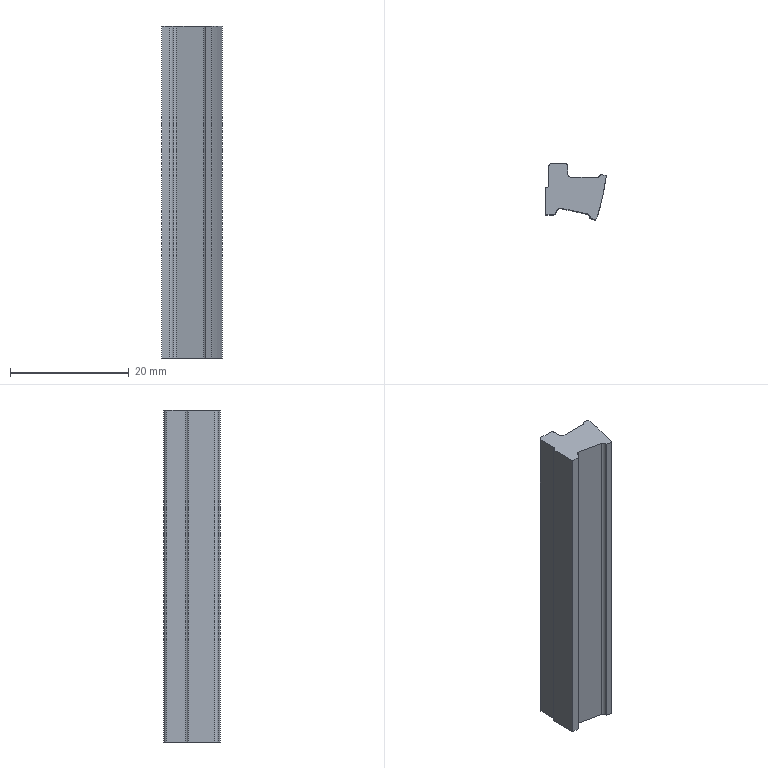Part | NX | features BREP 2 | 2 solids | 46 faces | box 10.188 x 9.472 x 56 mm | volume 7217 mm3 | plane 24 | cylinder 22 | commonest cylinder face diameters 1 x16 72.496 x2 72.701 x2 188.049 x2
STEP:
#1=CARTESIAN_POINT('',(5.069,2.402,-4.));
#2=VERTEX_POINT('',#1);
#3=CARTESIAN_POINT('',(5.069,2.402,52.));
#4=VERTEX_POINT('',#3);
#5=CARTESIAN_POINT('',(5.069,2.402,-4.));
#6=CARTESIAN_POINT('',(5.069,2.402,14.667));
#7=CARTESIAN_POINT('',(5.069,2.402,33.333));
#8=CARTESIAN_POINT('',(5.069,2.402,52.));
#9=B_SPLINE_CURVE_WITH_KNOTS('',3,(#5,#6,#7,#8),.UNSPECIFIED.,.F.,.F.,(4,4),(0.,1.),.UNSPECIFIED.);
#10=EDGE_CURVE('',#2,#4,#9,.T.);
#11=ORIENTED_EDGE('',*,*,#10,.T.);
#12=CARTESIAN_POINT('',(3.669,-3.886,52.));
#13=VERTEX_POINT('',#12);
#14=CARTESIAN_POINT('',(-30.974,7.123,52.));
#15=DIRECTION('',(0.,0.,1.));
#16=DIRECTION('',(1.,0.,0.));
#17=AXIS2_PLACEMENT_3D('',#14,#15,#16);
#18=CIRCLE('',#17,36.35);
#19=EDGE_CURVE('',#13,#4,#18,.T.);
#20=ORIENTED_EDGE('',*,*,#19,.F.);
#21=CARTESIAN_POINT('',(3.669,-3.886,-4.));
#22=VERTEX_POINT('',#21);
#23=CARTESIAN_POINT('',(3.669,-3.886,0.));
#24=DIRECTION('',(0.,0.,1.));
#25=VECTOR('',#24,1000.);
#26=LINE('',#23,#25);
#27=EDGE_CURVE('',#22,#13,#26,.T.);
#28=ORIENTED_EDGE('',*,*,#27,.F.);
#29=CARTESIAN_POINT('',(-30.974,7.123,-4.));
#30=DIRECTION('',(0.,0.,1.));
#31=DIRECTION('',(1.,0.,0.));
#32=AXIS2_PLACEMENT_3D('',#29,#30,#31);
#33=CIRCLE('',#32,36.35);
#34=EDGE_CURVE('',#22,#2,#33,.T.);
#35=ORIENTED_EDGE('',*,*,#34,.T.);
#36=EDGE_LOOP('',(#11,#20,#28,#35));
#37=FACE_BOUND('',#36,.T.);
#38=CARTESIAN_POINT('',(-30.974,7.123,0.));
#39=DIRECTION('',(0.,0.,1.));
#40=DIRECTION('',(-1.,0.,0.));
#41=AXIS2_PLACEMENT_3D('',#38,#39,#40);
#42=CYLINDRICAL_SURFACE('',#41,36.35);
#43=ADVANCED_FACE('',(#37),#42,.T.);
#44=ORIENTED_EDGE('',*,*,#27,.T.);
#45=CARTESIAN_POINT('',(3.379,-4.761,52.));
#46=VERTEX_POINT('',#45);
#47=CARTESIAN_POINT('',(-30.874,7.1,52.));
#48=DIRECTION('',(0.,0.,1.));
#49=DIRECTION('',(1.,0.,0.));
#50=AXIS2_PLACEMENT_3D('',#47,#48,#49);
#51=CIRCLE('',#50,36.248);
#52=EDGE_CURVE('',#46,#13,#51,.T.);
#53=ORIENTED_EDGE('',*,*,#52,.F.);
#54=CARTESIAN_POINT('',(3.379,-4.761,-4.));
#55=VERTEX_POINT('',#54);
#56=CARTESIAN_POINT('',(3.379,-4.761,0.));
#57=DIRECTION('',(0.,0.,1.));
#58=VECTOR('',#57,1000.);
#59=LINE('',#56,#58);
#60=EDGE_CURVE('',#55,#46,#59,.T.);
#61=ORIENTED_EDGE('',*,*,#60,.F.);
#62=CARTESIAN_POINT('',(-30.874,7.1,-4.));
#63=DIRECTION('',(0.,0.,1.));
#64=DIRECTION('',(1.,0.,0.));
#65=AXIS2_PLACEMENT_3D('',#62,#63,#64);
#66=CIRCLE('',#65,36.248);
#67=EDGE_CURVE('',#55,#22,#66,.T.);
#68=ORIENTED_EDGE('',*,*,#67,.T.);
#69=EDGE_LOOP('',(#44,#53,#61,#68));
#70=FACE_BOUND('',#69,.T.);
#71=CARTESIAN_POINT('',(-30.874,7.1,0.));
#72=DIRECTION('',(0.,0.,1.));
#73=DIRECTION('',(-1.,0.,0.));
#74=AXIS2_PLACEMENT_3D('',#71,#72,#73);
#75=CYLINDRICAL_SURFACE('',#74,36.248);
#76=ADVANCED_FACE('',(#70),#75,.T.);
#77=ORIENTED_EDGE('',*,*,#60,.T.);
#78=CARTESIAN_POINT('',(2.35,-4.418,52.));
#79=VERTEX_POINT('',#78);
#80=CARTESIAN_POINT('',(-11.943,0.3475,52.));
#81=DIRECTION('',(0.9487,-0.3163,0.));
#82=VECTOR('',#81,1000.);
#83=LINE('',#80,#82);
#84=EDGE_CURVE('',#79,#46,#83,.T.);
#85=ORIENTED_EDGE('',*,*,#84,.F.);
#86=CARTESIAN_POINT('',(2.35,-4.418,-4.));
#87=VERTEX_POINT('',#86);
#88=CARTESIAN_POINT('',(2.35,-4.418,0.));
#89=DIRECTION('',(0.,0.,1.));
#90=VECTOR('',#89,1000.);
#91=LINE('',#88,#90);
#92=EDGE_CURVE('',#87,#79,#91,.T.);
#93=ORIENTED_EDGE('',*,*,#92,.F.);
#94=CARTESIAN_POINT('',(-11.943,0.3475,-4.));
#95=DIRECTION('',(0.9487,-0.3163,0.));
#96=VECTOR('',#95,1000.);
#97=LINE('',#94,#96);
#98=EDGE_CURVE('',#87,#55,#97,.T.);
#99=ORIENTED_EDGE('',*,*,#98,.T.);
#100=EDGE_LOOP('',(#77,#85,#93,#99));
#101=FACE_BOUND('',#100,.T.);
#102=CARTESIAN_POINT('',(-11.943,0.3475,0.));
#103=DIRECTION('',(-0.3163,-0.9487,0.));
#104=DIRECTION('',(-0.9487,0.3163,0.));
#105=AXIS2_PLACEMENT_3D('',#102,#103,#104);
#106=PLANE('',#105);
#107=ADVANCED_FACE('',(#101),#106,.T.);
#108=ORIENTED_EDGE('',*,*,#92,.T.);
#109=CARTESIAN_POINT('',(1.98,-3.771,52.));
#110=VERTEX_POINT('',#109);
#111=CARTESIAN_POINT('',(1.876,-4.26,52.));
#112=DIRECTION('',(0.,0.,-1.));
#113=DIRECTION('',(1.,0.,0.));
#114=AXIS2_PLACEMENT_3D('',#111,#112,#113);
#115=CIRCLE('',#114,0.5);
#116=EDGE_CURVE('',#110,#79,#115,.T.);
#117=ORIENTED_EDGE('',*,*,#116,.F.);
#118=CARTESIAN_POINT('',(1.98,-3.771,-4.));
#119=VERTEX_POINT('',#118);
#120=CARTESIAN_POINT('',(1.98,-3.771,0.));
#121=DIRECTION('',(0.,0.,1.));
#122=VECTOR('',#121,1000.);
#123=LINE('',#120,#122);
#124=EDGE_CURVE('',#119,#110,#123,.T.);
#125=ORIENTED_EDGE('',*,*,#124,.F.);
#126=CARTESIAN_POINT('',(1.876,-4.26,-4.));
#127=DIRECTION('',(0.,0.,-1.));
#128=DIRECTION('',(1.,0.,0.));
#129=AXIS2_PLACEMENT_3D('',#126,#127,#128);
#130=CIRCLE('',#129,0.5);
#131=EDGE_CURVE('',#119,#87,#130,.T.);
#132=ORIENTED_EDGE('',*,*,#131,.T.);
#133=EDGE_LOOP('',(#108,#117,#125,#132));
#134=FACE_BOUND('',#133,.T.);
#135=CARTESIAN_POINT('',(1.876,-4.26,0.));
#136=DIRECTION('',(0.,0.,1.));
#137=DIRECTION('',(-1.,0.,0.));
#138=AXIS2_PLACEMENT_3D('',#135,#136,#137);
#139=CYLINDRICAL_SURFACE('',#138,0.5);
#140=ADVANCED_FACE('',(#134),#139,.F.);
#141=ORIENTED_EDGE('',*,*,#124,.T.);
#142=CARTESIAN_POINT('',(-2.566,-2.804,52.));
#143=VERTEX_POINT('',#142);
#144=CARTESIAN_POINT('',(1.98,-3.771,52.));
#145=DIRECTION('',(0.9781,-0.2079,0.));
#146=VECTOR('',#145,1000.);
#147=LINE('',#144,#146);
#148=EDGE_CURVE('',#143,#110,#147,.T.);
#149=ORIENTED_EDGE('',*,*,#148,.F.);
#150=CARTESIAN_POINT('',(-2.566,-2.804,-4.));
#151=VERTEX_POINT('',#150);
#152=CARTESIAN_POINT('',(-2.566,-2.804,0.));
#153=DIRECTION('',(0.,0.,1.));
#154=VECTOR('',#153,1000.);
#155=LINE('',#152,#154);
#156=EDGE_CURVE('',#151,#143,#155,.T.);
#157=ORIENTED_EDGE('',*,*,#156,.F.);
#158=CARTESIAN_POINT('',(1.98,-3.771,-4.));
#159=DIRECTION('',(0.9781,-0.2079,0.));
#160=VECTOR('',#159,1000.);
#161=LINE('',#158,#160);
#162=EDGE_CURVE('',#151,#119,#161,.T.);
#163=ORIENTED_EDGE('',*,*,#162,.T.);
#164=EDGE_LOOP('',(#141,#149,#157,#163));
#165=FACE_BOUND('',#164,.T.);
#166=CARTESIAN_POINT('',(1.98,-3.771,0.));
#167=DIRECTION('',(0.2079,0.9781,0.));
#168=DIRECTION('',(0.9781,-0.2079,0.));
#169=AXIS2_PLACEMENT_3D('',#166,#167,#168);
#170=PLANE('',#169);
#171=ADVANCED_FACE('',(#165),#170,.F.);
#172=ORIENTED_EDGE('',*,*,#156,.T.);
#173=CARTESIAN_POINT('',(-3.123,-3.082,52.));
#174=VERTEX_POINT('',#173);
#175=CARTESIAN_POINT('',(-2.67,-3.294,52.));
#176=DIRECTION('',(0.,0.,-1.));
#177=DIRECTION('',(1.,0.,0.));
#178=AXIS2_PLACEMENT_3D('',#175,#176,#177);
#179=CIRCLE('',#178,0.5);
#180=EDGE_CURVE('',#174,#143,#179,.T.);
#181=ORIENTED_EDGE('',*,*,#180,.F.);
#182=CARTESIAN_POINT('',(-3.123,-3.082,-4.));
#183=VERTEX_POINT('',#182);
#184=CARTESIAN_POINT('',(-3.123,-3.082,0.));
#185=DIRECTION('',(0.,0.,1.));
#186=VECTOR('',#185,1000.);
#187=LINE('',#184,#186);
#188=EDGE_CURVE('',#183,#174,#187,.T.);
#189=ORIENTED_EDGE('',*,*,#188,.F.);
#190=CARTESIAN_POINT('',(-2.67,-3.294,-4.));
#191=DIRECTION('',(0.,0.,-1.));
#192=DIRECTION('',(1.,0.,0.));
#193=AXIS2_PLACEMENT_3D('',#190,#191,#192);
#194=CIRCLE('',#193,0.5);
#195=EDGE_CURVE('',#183,#151,#194,.T.);
#196=ORIENTED_EDGE('',*,*,#195,.T.);
#197=EDGE_LOOP('',(#172,#181,#189,#196));
#198=FACE_BOUND('',#197,.T.);
#199=CARTESIAN_POINT('',(-2.67,-3.294,0.));
#200=DIRECTION('',(0.,0.,1.));
#201=DIRECTION('',(-1.,0.,0.));
#202=AXIS2_PLACEMENT_3D('',#199,#200,#201);
#203=CYLINDRICAL_SURFACE('',#202,0.5);
#204=ADVANCED_FACE('',(#198),#203,.F.);
#205=ORIENTED_EDGE('',*,*,#188,.T.);
#206=CARTESIAN_POINT('',(-3.37,-3.611,52.));
#207=VERTEX_POINT('',#206);
#208=CARTESIAN_POINT('',(-3.123,-3.082,52.));
#209=DIRECTION('',(0.4226,0.9063,0.));
#210=VECTOR('',#209,1000.);
#211=LINE('',#208,#210);
#212=EDGE_CURVE('',#207,#174,#211,.T.);
#213=ORIENTED_EDGE('',*,*,#212,.F.);
#214=CARTESIAN_POINT('',(-3.37,-3.611,-4.));
#215=VERTEX_POINT('',#214);
#216=CARTESIAN_POINT('',(-3.37,-3.611,0.));
#217=DIRECTION('',(0.,0.,1.));
#218=VECTOR('',#217,1000.);
#219=LINE('',#216,#218);
#220=EDGE_CURVE('',#215,#207,#219,.T.);
#221=ORIENTED_EDGE('',*,*,#220,.F.);
#222=CARTESIAN_POINT('',(-3.123,-3.082,-4.));
#223=DIRECTION('',(0.4226,0.9063,0.));
#224=VECTOR('',#223,1000.);
#225=LINE('',#222,#224);
#226=EDGE_CURVE('',#215,#183,#225,.T.);
#227=ORIENTED_EDGE('',*,*,#226,.T.);
#228=EDGE_LOOP('',(#205,#213,#221,#227));
#229=FACE_BOUND('',#228,.T.);
#230=CARTESIAN_POINT('',(-3.123,-3.082,0.));
#231=DIRECTION('',(-0.9063,0.4226,0.));
#232=DIRECTION('',(0.4226,0.9063,0.));
#233=AXIS2_PLACEMENT_3D('',#230,#231,#232);
#234=PLANE('',#233);
#235=ADVANCED_FACE('',(#229),#234,.F.);
#236=ORIENTED_EDGE('',*,*,#220,.T.);
#237=CARTESIAN_POINT('',(-3.823,-3.9,52.));
#238=VERTEX_POINT('',#237);
#239=CARTESIAN_POINT('',(-3.823,-3.4,52.));
#240=DIRECTION('',(0.,0.,1.));
#241=DIRECTION('',(1.,0.,0.));
#242=AXIS2_PLACEMENT_3D('',#239,#240,#241);
#243=CIRCLE('',#242,0.5);
#244=EDGE_CURVE('',#238,#207,#243,.T.);
#245=ORIENTED_EDGE('',*,*,#244,.F.);
#246=CARTESIAN_POINT('',(-3.823,-3.9,-4.));
#247=VERTEX_POINT('',#246);
#248=CARTESIAN_POINT('',(-3.823,-3.9,0.));
#249=DIRECTION('',(0.,0.,1.));
#250=VECTOR('',#249,1000.);
#251=LINE('',#248,#250);
#252=EDGE_CURVE('',#247,#238,#251,.T.);
#253=ORIENTED_EDGE('',*,*,#252,.F.);
#254=CARTESIAN_POINT('',(-3.823,-3.4,-4.));
#255=DIRECTION('',(0.,0.,1.));
#256=DIRECTION('',(1.,0.,0.));
#257=AXIS2_PLACEMENT_3D('',#254,#255,#256);
#258=CIRCLE('',#257,0.5);
#259=EDGE_CURVE('',#247,#215,#258,.T.);
#260=ORIENTED_EDGE('',*,*,#259,.T.);
#261=EDGE_LOOP('',(#236,#245,#253,#260));
#262=FACE_BOUND('',#261,.T.);
#263=CARTESIAN_POINT('',(-3.823,-3.4,0.));
#264=DIRECTION('',(0.,0.,1.));
#265=DIRECTION('',(-1.,0.,0.));
#266=AXIS2_PLACEMENT_3D('',#263,#264,#265);
#267=CYLINDRICAL_SURFACE('',#266,0.5);
#268=ADVANCED_FACE('',(#262),#267,.T.);
#269=ORIENTED_EDGE('',*,*,#252,.T.);
#270=CARTESIAN_POINT('',(-5.087,-3.9,52.));
#271=VERTEX_POINT('',#270);
#272=CARTESIAN_POINT('',(-7.561,-3.9,52.));
#273=DIRECTION('',(1.,0.,0.));
#274=VECTOR('',#273,1000.);
#275=LINE('',#272,#274);
#276=EDGE_CURVE('',#271,#238,#275,.T.);
#277=ORIENTED_EDGE('',*,*,#276,.F.);
#278=CARTESIAN_POINT('',(-5.087,-3.9,-4.));
#279=VERTEX_POINT('',#278);
#280=CARTESIAN_POINT('',(-5.087,-3.9,0.));
#281=DIRECTION('',(0.,0.,1.));
#282=VECTOR('',#281,1000.);
#283=LINE('',#280,#282);
#284=EDGE_CURVE('',#279,#271,#283,.T.);
#285=ORIENTED_EDGE('',*,*,#284,.F.);
#286=CARTESIAN_POINT('',(-7.561,-3.9,-4.));
#287=DIRECTION('',(1.,0.,0.));
#288=VECTOR('',#287,1000.);
#289=LINE('',#286,#288);
#290=EDGE_CURVE('',#279,#247,#289,.T.);
#291=ORIENTED_EDGE('',*,*,#290,.T.);
#292=EDGE_LOOP('',(#269,#277,#285,#291));
#293=FACE_BOUND('',#292,.T.);
#294=CARTESIAN_POINT('',(-3.823,-3.9,0.));
#295=DIRECTION('',(0.,1.,0.));
#296=DIRECTION('',(1.,0.,0.));
#297=AXIS2_PLACEMENT_3D('',#294,#295,#296);
#298=PLANE('',#297);
#299=ADVANCED_FACE('',(#293),#298,.F.);
#300=ORIENTED_EDGE('',*,*,#284,.T.);
#301=CARTESIAN_POINT('',(-5.087,0.6109,52.));
#302=VERTEX_POINT('',#301);
#303=CARTESIAN_POINT('',(-5.087,13.492,52.));
#304=DIRECTION('',(0.,-1.,0.));
#305=VECTOR('',#304,1000.);
#306=LINE('',#303,#305);
#307=EDGE_CURVE('',#302,#271,#306,.T.);
#308=ORIENTED_EDGE('',*,*,#307,.F.);
#309=CARTESIAN_POINT('',(-5.087,0.6109,-4.));
#310=VERTEX_POINT('',#309);
#311=CARTESIAN_POINT('',(-5.087,0.6109,0.));
#312=DIRECTION('',(0.,0.,1.));
#313=VECTOR('',#312,1000.);
#314=LINE('',#311,#313);
#315=EDGE_CURVE('',#310,#302,#314,.T.);
#316=ORIENTED_EDGE('',*,*,#315,.F.);
#317=CARTESIAN_POINT('',(-5.087,13.492,-4.));
#318=DIRECTION('',(0.,-1.,0.));
#319=VECTOR('',#318,1000.);
#320=LINE('',#317,#319);
#321=EDGE_CURVE('',#310,#279,#320,.T.);
#322=ORIENTED_EDGE('',*,*,#321,.T.);
#323=EDGE_LOOP('',(#300,#308,#316,#322));
#324=FACE_BOUND('',#323,.T.);
#325=CARTESIAN_POINT('',(-5.087,13.492,0.));
#326=DIRECTION('',(-1.,0.,0.));
#327=DIRECTION('',(0.,1.,0.));
#328=AXIS2_PLACEMENT_3D('',#325,#326,#327);
#329=PLANE('',#328);
#330=ADVANCED_FACE('',(#324),#329,.T.);
#331=ORIENTED_EDGE('',*,*,#315,.T.);
#332=CARTESIAN_POINT('',(-4.587,1.111,52.));
#333=VERTEX_POINT('',#332);
#334=CARTESIAN_POINT('',(-5.087,1.111,52.));
#335=DIRECTION('',(0.,0.,-1.));
#336=DIRECTION('',(1.,0.,0.));
#337=AXIS2_PLACEMENT_3D('',#334,#335,#336);
#338=CIRCLE('',#337,0.5);
#339=EDGE_CURVE('',#333,#302,#338,.T.);
#340=ORIENTED_EDGE('',*,*,#339,.F.);
#341=CARTESIAN_POINT('',(-4.587,1.111,-4.));
#342=VERTEX_POINT('',#341);
#343=CARTESIAN_POINT('',(-4.587,1.111,0.));
#344=DIRECTION('',(0.,0.,1.));
#345=VECTOR('',#344,1000.);
#346=LINE('',#343,#345);
#347=EDGE_CURVE('',#342,#333,#346,.T.);
#348=ORIENTED_EDGE('',*,*,#347,.F.);
#349=CARTESIAN_POINT('',(-5.087,1.111,-4.));
#350=DIRECTION('',(0.,0.,-1.));
#351=DIRECTION('',(1.,0.,0.));
#352=AXIS2_PLACEMENT_3D('',#349,#350,#351);
#353=CIRCLE('',#352,0.5);
#354=EDGE_CURVE('',#342,#310,#353,.T.);
#355=ORIENTED_EDGE('',*,*,#354,.T.);
#356=EDGE_LOOP('',(#331,#340,#348,#355));
#357=FACE_BOUND('',#356,.T.);
#358=CARTESIAN_POINT('',(-5.087,1.111,0.));
#359=DIRECTION('',(0.,0.,1.));
#360=DIRECTION('',(-1.,0.,0.));
#361=AXIS2_PLACEMENT_3D('',#358,#359,#360);
#362=CYLINDRICAL_SURFACE('',#361,0.5);
#363=ADVANCED_FACE('',(#357),#362,.F.);
#364=ORIENTED_EDGE('',*,*,#347,.T.);
#365=CARTESIAN_POINT('',(-4.587,4.211,52.));
#366=VERTEX_POINT('',#365);
#367=CARTESIAN_POINT('',(-4.587,13.492,52.));
#368=DIRECTION('',(0.,-1.,0.));
#369=VECTOR('',#368,1000.);
#370=LINE('',#367,#369);
#371=EDGE_CURVE('',#366,#333,#370,.T.);
#372=ORIENTED_EDGE('',*,*,#371,.F.);
#373=CARTESIAN_POINT('',(-4.587,4.211,-4.));
#374=VERTEX_POINT('',#373);
#375=CARTESIAN_POINT('',(-4.587,4.211,0.));
#376=DIRECTION('',(0.,0.,1.));
#377=VECTOR('',#376,1000.);
#378=LINE('',#375,#377);
#379=EDGE_CURVE('',#374,#366,#378,.T.);
#380=ORIENTED_EDGE('',*,*,#379,.F.);
#381=CARTESIAN_POINT('',(-4.587,13.492,-4.));
#382=DIRECTION('',(0.,-1.,0.));
#383=VECTOR('',#382,1000.);
#384=LINE('',#381,#383);
#385=EDGE_CURVE('',#374,#342,#384,.T.);
#386=ORIENTED_EDGE('',*,*,#385,.T.);
#387=EDGE_LOOP('',(#364,#372,#380,#386));
#388=FACE_BOUND('',#387,.T.);
#389=CARTESIAN_POINT('',(-4.587,1.111,0.));
#390=DIRECTION('',(1.,0.,0.));
#391=DIRECTION('',(0.,-1.,0.));
#392=AXIS2_PLACEMENT_3D('',#389,#390,#391);
#393=PLANE('',#392);
#394=ADVANCED_FACE('',(#388),#393,.F.);
#395=ORIENTED_EDGE('',*,*,#379,.T.);
#396=CARTESIAN_POINT('',(-4.087,4.711,52.));
#397=VERTEX_POINT('',#396);
#398=CARTESIAN_POINT('',(-4.087,4.211,52.));
#399=DIRECTION('',(0.,0.,1.));
#400=DIRECTION('',(1.,0.,0.));
#401=AXIS2_PLACEMENT_3D('',#398,#399,#400);
#402=CIRCLE('',#401,0.5);
#403=EDGE_CURVE('',#397,#366,#402,.T.);
#404=ORIENTED_EDGE('',*,*,#403,.F.);
#405=CARTESIAN_POINT('',(-4.087,4.711,-4.));
#406=VERTEX_POINT('',#405);
#407=CARTESIAN_POINT('',(-4.087,4.711,0.));
#408=DIRECTION('',(0.,0.,1.));
#409=VECTOR('',#408,1000.);
#410=LINE('',#407,#409);
#411=EDGE_CURVE('',#406,#397,#410,.T.);
#412=ORIENTED_EDGE('',*,*,#411,.F.);
#413=CARTESIAN_POINT('',(-4.087,4.211,-4.));
#414=DIRECTION('',(0.,0.,1.));
#415=DIRECTION('',(1.,0.,0.));
#416=AXIS2_PLACEMENT_3D('',#413,#414,#415);
#417=CIRCLE('',#416,0.5);
#418=EDGE_CURVE('',#406,#374,#417,.T.);
#419=ORIENTED_EDGE('',*,*,#418,.T.);
#420=EDGE_LOOP('',(#395,#404,#412,#419));
#421=FACE_BOUND('',#420,.T.);
#422=CARTESIAN_POINT('',(-4.087,4.211,0.));
#423=DIRECTION('',(0.,0.,1.));
#424=DIRECTION('',(-1.,0.,0.));
#425=AXIS2_PLACEMENT_3D('',#422,#423,#424);
#426=CYLINDRICAL_SURFACE('',#425,0.5);
#427=ADVANCED_FACE('',(#421),#426,.T.);
#428=ORIENTED_EDGE('',*,*,#411,.T.);
#429=CARTESIAN_POINT('',(-1.887,4.711,52.));
#430=VERTEX_POINT('',#429);
#431=CARTESIAN_POINT('',(-7.561,4.711,52.));
#432=DIRECTION('',(-1.,0.,0.));
#433=VECTOR('',#432,1000.);
#434=LINE('',#431,#433);
#435=EDGE_CURVE('',#430,#397,#434,.T.);
#436=ORIENTED_EDGE('',*,*,#435,.F.);
#437=CARTESIAN_POINT('',(-1.887,4.711,-4.));
#438=VERTEX_POINT('',#437);
#439=CARTESIAN_POINT('',(-1.887,4.711,0.));
#440=DIRECTION('',(0.,0.,1.));
#441=VECTOR('',#440,1000.);
#442=LINE('',#439,#441);
#443=EDGE_CURVE('',#438,#430,#442,.T.);
#444=ORIENTED_EDGE('',*,*,#443,.F.);
#445=CARTESIAN_POINT('',(-7.561,4.711,-4.));
#446=DIRECTION('',(-1.,0.,0.));
#447=VECTOR('',#446,1000.);
#448=LINE('',#445,#447);
#449=EDGE_CURVE('',#438,#406,#448,.T.);
#450=ORIENTED_EDGE('',*,*,#449,.T.);
#451=EDGE_LOOP('',(#428,#436,#444,#450));
#452=FACE_BOUND('',#451,.T.);
#453=CARTESIAN_POINT('',(-4.087,4.711,0.));
#454=DIRECTION('',(0.,-1.,0.));
#455=DIRECTION('',(-1.,0.,0.));
#456=AXIS2_PLACEMENT_3D('',#453,#454,#455);
#457=PLANE('',#456);
#458=ADVANCED_FACE('',(#452),#457,.F.);
#459=ORIENTED_EDGE('',*,*,#443,.T.);
#460=CARTESIAN_POINT('',(-1.387,4.211,52.));
#461=VERTEX_POINT('',#460);
#462=CARTESIAN_POINT('',(-1.887,4.211,52.));
#463=DIRECTION('',(0.,0.,1.));
#464=DIRECTION('',(1.,0.,0.));
#465=AXIS2_PLACEMENT_3D('',#462,#463,#464);
#466=CIRCLE('',#465,0.5);
#467=EDGE_CURVE('',#461,#430,#466,.T.);
#468=ORIENTED_EDGE('',*,*,#467,.F.);
#469=CARTESIAN_POINT('',(-1.387,4.211,-4.));
#470=VERTEX_POINT('',#469);
#471=CARTESIAN_POINT('',(-1.387,4.211,0.));
#472=DIRECTION('',(0.,0.,1.));
#473=VECTOR('',#472,1000.);
#474=LINE('',#471,#473);
#475=EDGE_CURVE('',#470,#461,#474,.T.);
#476=ORIENTED_EDGE('',*,*,#475,.F.);
#477=CARTESIAN_POINT('',(-1.887,4.211,-4.));
#478=DIRECTION('',(0.,0.,1.));
#479=DIRECTION('',(1.,0.,0.));
#480=AXIS2_PLACEMENT_3D('',#477,#478,#479);
#481=CIRCLE('',#480,0.5);
#482=EDGE_CURVE('',#470,#438,#481,.T.);
#483=ORIENTED_EDGE('',*,*,#482,.T.);
#484=EDGE_LOOP('',(#459,#468,#476,#483));
#485=FACE_BOUND('',#484,.T.);
#486=CARTESIAN_POINT('',(-1.887,4.211,0.));
#487=DIRECTION('',(0.,0.,1.));
#488=DIRECTION('',(-1.,0.,0.));
#489=AXIS2_PLACEMENT_3D('',#486,#487,#488);
#490=CYLINDRICAL_SURFACE('',#489,0.5);
#491=ADVANCED_FACE('',(#485),#490,.T.);
#492=ORIENTED_EDGE('',*,*,#475,.T.);
#493=CARTESIAN_POINT('',(-1.387,2.907,52.));
#494=VERTEX_POINT('',#493);
#495=CARTESIAN_POINT('',(-1.387,13.492,52.));
#496=DIRECTION('',(0.,1.,0.));
#497=VECTOR('',#496,1000.);
#498=LINE('',#495,#497);
#499=EDGE_CURVE('',#494,#461,#498,.T.);
#500=ORIENTED_EDGE('',*,*,#499,.F.);
#501=CARTESIAN_POINT('',(-1.387,2.907,-4.));
#502=VERTEX_POINT('',#501);
#503=CARTESIAN_POINT('',(-1.387,2.907,0.));
#504=DIRECTION('',(0.,0.,1.));
#505=VECTOR('',#504,1000.);
#506=LINE('',#503,#505);
#507=EDGE_CURVE('',#502,#494,#506,.T.);
#508=ORIENTED_EDGE('',*,*,#507,.F.);
#509=CARTESIAN_POINT('',(-1.387,13.492,-4.));
#510=DIRECTION('',(0.,1.,0.));
#511=VECTOR('',#510,1000.);
#512=LINE('',#509,#511);
#513=EDGE_CURVE('',#502,#470,#512,.T.);
#514=ORIENTED_EDGE('',*,*,#513,.T.);
#515=EDGE_LOOP('',(#492,#500,#508,#514));
#516=FACE_BOUND('',#515,.T.);
#517=CARTESIAN_POINT('',(-1.387,4.211,0.));
#518=DIRECTION('',(-1.,0.,0.));
#519=DIRECTION('',(0.,1.,0.));
#520=AXIS2_PLACEMENT_3D('',#517,#518,#519);
#521=PLANE('',#520);
#522=ADVANCED_FACE('',(#516),#521,.F.);
#523=ORIENTED_EDGE('',*,*,#507,.T.);
#524=CARTESIAN_POINT('',(-0.8868,2.407,52.));
#525=VERTEX_POINT('',#524);
#526=CARTESIAN_POINT('',(-0.8868,2.907,52.));
#527=DIRECTION('',(0.,0.,-1.));
#528=DIRECTION('',(1.,0.,0.));
#529=AXIS2_PLACEMENT_3D('',#526,#527,#528);
#530=CIRCLE('',#529,0.5);
#531=EDGE_CURVE('',#525,#494,#530,.T.);
#532=ORIENTED_EDGE('',*,*,#531,.F.);
#533=CARTESIAN_POINT('',(-0.8868,2.407,-4.));
#534=VERTEX_POINT('',#533);
#535=CARTESIAN_POINT('',(-0.8868,2.407,0.));
#536=DIRECTION('',(0.,0.,1.));
#537=VECTOR('',#536,1000.);
#538=LINE('',#535,#537);
#539=EDGE_CURVE('',#534,#525,#538,.T.);
#540=ORIENTED_EDGE('',*,*,#539,.F.);
#541=CARTESIAN_POINT('',(-0.8868,2.907,-4.));
#542=DIRECTION('',(0.,0.,-1.));
#543=DIRECTION('',(1.,0.,0.));
#544=AXIS2_PLACEMENT_3D('',#541,#542,#543);
#545=CIRCLE('',#544,0.5);
#546=EDGE_CURVE('',#534,#502,#545,.T.);
#547=ORIENTED_EDGE('',*,*,#546,.T.);
#548=EDGE_LOOP('',(#523,#532,#540,#547));
#549=FACE_BOUND('',#548,.T.);
#550=CARTESIAN_POINT('',(-0.8868,2.907,0.));
#551=DIRECTION('',(0.,0.,1.));
#552=DIRECTION('',(-1.,0.,0.));
#553=AXIS2_PLACEMENT_3D('',#550,#551,#552);
#554=CYLINDRICAL_SURFACE('',#553,0.5);
#555=ADVANCED_FACE('',(#549),#554,.F.);
#556=ORIENTED_EDGE('',*,*,#539,.T.);
#557=CARTESIAN_POINT('',(3.623,2.407,52.));
#558=VERTEX_POINT('',#557);
#559=CARTESIAN_POINT('',(-7.561,2.407,52.));
#560=DIRECTION('',(-1.,0.,0.));
#561=VECTOR('',#560,1000.);
#562=LINE('',#559,#561);
#563=EDGE_CURVE('',#558,#525,#562,.T.);
#564=ORIENTED_EDGE('',*,*,#563,.F.);
#565=CARTESIAN_POINT('',(3.623,2.407,-4.));
#566=VERTEX_POINT('',#565);
#567=CARTESIAN_POINT('',(3.623,2.407,0.));
#568=DIRECTION('',(0.,0.,1.));
#569=VECTOR('',#568,1000.);
#570=LINE('',#567,#569);
#571=EDGE_CURVE('',#566,#558,#570,.T.);
#572=ORIENTED_EDGE('',*,*,#571,.F.);
#573=CARTESIAN_POINT('',(-7.561,2.407,-4.));
#574=DIRECTION('',(-1.,0.,0.));
#575=VECTOR('',#574,1000.);
#576=LINE('',#573,#575);
#577=EDGE_CURVE('',#566,#534,#576,.T.);
#578=ORIENTED_EDGE('',*,*,#577,.T.);
#579=EDGE_LOOP('',(#556,#564,#572,#578));
#580=FACE_BOUND('',#579,.T.);
#581=CARTESIAN_POINT('',(-0.8868,2.407,0.));
#582=DIRECTION('',(0.,-1.,0.));
#583=DIRECTION('',(-1.,0.,0.));
#584=AXIS2_PLACEMENT_3D('',#581,#582,#583);
#585=PLANE('',#584);
#586=ADVANCED_FACE('',(#580),#585,.F.);
#587=ORIENTED_EDGE('',*,*,#571,.T.);
#588=CARTESIAN_POINT('',(4.12,2.852,52.));
#589=VERTEX_POINT('',#588);
#590=CARTESIAN_POINT('',(3.623,2.907,52.));
#591=DIRECTION('',(0.,0.,-1.));
#592=DIRECTION('',(1.,0.,0.));
#593=AXIS2_PLACEMENT_3D('',#590,#591,#592);
#594=CIRCLE('',#593,0.5);
#595=EDGE_CURVE('',#589,#558,#594,.T.);
#596=ORIENTED_EDGE('',*,*,#595,.F.);
#597=CARTESIAN_POINT('',(4.12,2.852,-4.));
#598=VERTEX_POINT('',#597);
#599=CARTESIAN_POINT('',(4.12,2.852,0.));
#600=DIRECTION('',(0.,0.,1.));
#601=VECTOR('',#600,1000.);
#602=LINE('',#599,#601);
#603=EDGE_CURVE('',#598,#589,#602,.T.);
#604=ORIENTED_EDGE('',*,*,#603,.F.);
#605=CARTESIAN_POINT('',(3.623,2.907,-4.));
#606=DIRECTION('',(0.,0.,-1.));
#607=DIRECTION('',(1.,0.,0.));
#608=AXIS2_PLACEMENT_3D('',#605,#606,#607);
#609=CIRCLE('',#608,0.5);
#610=EDGE_CURVE('',#598,#566,#609,.T.);
#611=ORIENTED_EDGE('',*,*,#610,.T.);
#612=EDGE_LOOP('',(#587,#596,#604,#611));
#613=FACE_BOUND('',#612,.T.);
#614=CARTESIAN_POINT('',(3.623,2.907,0.));
#615=DIRECTION('',(0.,0.,1.));
#616=DIRECTION('',(-1.,0.,0.));
#617=AXIS2_PLACEMENT_3D('',#614,#615,#616);
#618=CYLINDRICAL_SURFACE('',#617,0.5);
#619=ADVANCED_FACE('',(#613),#618,.F.);
#620=ORIENTED_EDGE('',*,*,#603,.T.);
#621=CARTESIAN_POINT('',(5.101,2.743,52.));
#622=VERTEX_POINT('',#621);
#623=CARTESIAN_POINT('',(-8.587,4.265,52.));
#624=DIRECTION('',(-0.9939,0.1105,0.));
#625=VECTOR('',#624,1000.);
#626=LINE('',#623,#625);
#627=EDGE_CURVE('',#622,#589,#626,.T.);
#628=ORIENTED_EDGE('',*,*,#627,.F.);
#629=CARTESIAN_POINT('',(5.101,2.743,-4.));
#630=VERTEX_POINT('',#629);
#631=CARTESIAN_POINT('',(5.101,2.743,0.));
#632=DIRECTION('',(0.,0.,1.));
#633=VECTOR('',#632,1000.);
#634=LINE('',#631,#633);
#635=EDGE_CURVE('',#630,#622,#634,.T.);
#636=ORIENTED_EDGE('',*,*,#635,.F.);
#637=CARTESIAN_POINT('',(-8.587,4.265,-4.));
#638=DIRECTION('',(-0.9939,0.1105,0.));
#639=VECTOR('',#638,1000.);
#640=LINE('',#637,#639);
#641=EDGE_CURVE('',#630,#598,#640,.T.);
#642=ORIENTED_EDGE('',*,*,#641,.T.);
#643=EDGE_LOOP('',(#620,#628,#636,#642));
#644=FACE_BOUND('',#643,.T.);
#645=CARTESIAN_POINT('',(-8.587,4.265,0.));
#646=DIRECTION('',(-0.1105,-0.9939,0.));
#647=DIRECTION('',(-0.9939,0.1105,0.));
#648=AXIS2_PLACEMENT_3D('',#645,#646,#647);
#649=PLANE('',#648);
#650=ADVANCED_FACE('',(#644),#649,.F.);
#651=CARTESIAN_POINT('',(-88.525,11.396,-4.));
#652=DIRECTION('',(0.,0.,1.));
#653=DIRECTION('',(1.,0.,0.));
#654=AXIS2_PLACEMENT_3D('',#651,#652,#653);
#655=CIRCLE('',#654,94.024);
#656=EDGE_CURVE('',#2,#630,#655,.T.);
#657=ORIENTED_EDGE('',*,*,#656,.T.);
#658=ORIENTED_EDGE('',*,*,#635,.T.);
#659=CARTESIAN_POINT('',(-88.525,11.396,52.));
#660=DIRECTION('',(0.,0.,1.));
#661=DIRECTION('',(1.,0.,0.));
#662=AXIS2_PLACEMENT_3D('',#659,#660,#661);
#663=CIRCLE('',#662,94.024);
#664=EDGE_CURVE('',#4,#622,#663,.T.);
#665=ORIENTED_EDGE('',*,*,#664,.F.);
#666=ORIENTED_EDGE('',*,*,#10,.F.);
#667=EDGE_LOOP('',(#657,#658,#665,#666));
#668=FACE_BOUND('',#667,.T.);
#669=CARTESIAN_POINT('',(-88.525,11.396,0.));
#670=DIRECTION('',(0.,0.,1.));
#671=DIRECTION('',(-1.,0.,0.));
#672=AXIS2_PLACEMENT_3D('',#669,#670,#671);
#673=CYLINDRICAL_SURFACE('',#672,94.024);
#674=ADVANCED_FACE('',(#668),#673,.T.);
#675=ORIENTED_EDGE('',*,*,#627,.T.);
#676=ORIENTED_EDGE('',*,*,#595,.T.);
#677=ORIENTED_EDGE('',*,*,#563,.T.);
#678=ORIENTED_EDGE('',*,*,#531,.T.);
#679=ORIENTED_EDGE('',*,*,#499,.T.);
#680=ORIENTED_EDGE('',*,*,#467,.T.);
#681=ORIENTED_EDGE('',*,*,#435,.T.);
#682=ORIENTED_EDGE('',*,*,#403,.T.);
#683=ORIENTED_EDGE('',*,*,#371,.T.);
#684=ORIENTED_EDGE('',*,*,#339,.T.);
#685=ORIENTED_EDGE('',*,*,#307,.T.);
#686=ORIENTED_EDGE('',*,*,#276,.T.);
#687=ORIENTED_EDGE('',*,*,#244,.T.);
#688=ORIENTED_EDGE('',*,*,#212,.T.);
#689=ORIENTED_EDGE('',*,*,#180,.T.);
#690=ORIENTED_EDGE('',*,*,#148,.T.);
#691=ORIENTED_EDGE('',*,*,#116,.T.);
#692=ORIENTED_EDGE('',*,*,#84,.T.);
#693=ORIENTED_EDGE('',*,*,#52,.T.);
#694=ORIENTED_EDGE('',*,*,#19,.T.);
#695=ORIENTED_EDGE('',*,*,#664,.T.);
#696=EDGE_LOOP('',(#675,#676,#677,#678,#679,#680,#681,#682,#683,#684,#685,#686,#687,#688,#689,#690,#691,#692,#693,#694,#695));
#697=FACE_BOUND('',#696,.T.);
#698=CARTESIAN_POINT('',(-7.561,13.492,52.));
#699=DIRECTION('',(0.,0.,1.));
#700=DIRECTION('',(-1.,0.,0.));
#701=AXIS2_PLACEMENT_3D('',#698,#699,#700);
#702=PLANE('',#701);
#703=ADVANCED_FACE('',(#697),#702,.T.);
#704=ORIENTED_EDGE('',*,*,#641,.F.);
#705=ORIENTED_EDGE('',*,*,#656,.F.);
#706=ORIENTED_EDGE('',*,*,#34,.F.);
#707=ORIENTED_EDGE('',*,*,#67,.F.);
#708=ORIENTED_EDGE('',*,*,#98,.F.);
#709=ORIENTED_EDGE('',*,*,#131,.F.);
#710=ORIENTED_EDGE('',*,*,#162,.F.);
#711=ORIENTED_EDGE('',*,*,#195,.F.);
#712=ORIENTED_EDGE('',*,*,#226,.F.);
#713=ORIENTED_EDGE('',*,*,#259,.F.);
#714=ORIENTED_EDGE('',*,*,#290,.F.);
#715=ORIENTED_EDGE('',*,*,#321,.F.);
#716=ORIENTED_EDGE('',*,*,#354,.F.);
#717=ORIENTED_EDGE('',*,*,#385,.F.);
#718=ORIENTED_EDGE('',*,*,#418,.F.);
#719=ORIENTED_EDGE('',*,*,#449,.F.);
#720=ORIENTED_EDGE('',*,*,#482,.F.);
#721=ORIENTED_EDGE('',*,*,#513,.F.);
#722=ORIENTED_EDGE('',*,*,#546,.F.);
#723=ORIENTED_EDGE('',*,*,#577,.F.);
#724=ORIENTED_EDGE('',*,*,#610,.F.);
#725=EDGE_LOOP('',(#704,#705,#706,#707,#708,#709,#710,#711,#712,#713,#714,#715,#716,#717,#718,#719,#720,#721,#722,#723,#724));
#726=FACE_BOUND('',#725,.T.);
#727=CARTESIAN_POINT('',(-7.561,13.492,-4.));
#728=DIRECTION('',(0.,0.,1.));
#729=DIRECTION('',(-1.,0.,0.));
#730=AXIS2_PLACEMENT_3D('',#727,#728,#729);
#731=PLANE('',#730);
#732=ADVANCED_FACE('',(#726),#731,.F.);
#733=CLOSED_SHELL('',(#43,#76,#107,#140,#171,#204,#235,#268,#299,#330,#363,#394,#427,#458,#491,#522,#555,#586,#619,#650,#674,#703,#732));
#734=MANIFOLD_SOLID_BREP('',#733);
#735=CARTESIAN_POINT('',(5.069,2.402,-4.));
#736=VERTEX_POINT('',#735);
#737=CARTESIAN_POINT('',(5.069,2.402,52.));
#738=VERTEX_POINT('',#737);
#739=CARTESIAN_POINT('',(5.069,2.402,-4.));
#740=CARTESIAN_POINT('',(5.069,2.402,14.667));
#741=CARTESIAN_POINT('',(5.069,2.402,33.333));
#742=CARTESIAN_POINT('',(5.069,2.402,52.));
#743=B_SPLINE_CURVE_WITH_KNOTS('',3,(#739,#740,#741,#742),.UNSPECIFIED.,.F.,.F.,(4,4),(0.,1.),.UNSPECIFIED.);
#744=EDGE_CURVE('',#736,#738,#743,.T.);
#745=ORIENTED_EDGE('',*,*,#744,.T.);
#746=CARTESIAN_POINT('',(3.669,-3.886,52.));
#747=VERTEX_POINT('',#746);
#748=CARTESIAN_POINT('',(-30.974,7.123,52.));
#749=DIRECTION('',(0.,0.,1.));
#750=DIRECTION('',(1.,0.,0.));
#751=AXIS2_PLACEMENT_3D('',#748,#749,#750);
#752=CIRCLE('',#751,36.35);
#753=EDGE_CURVE('',#747,#738,#752,.T.);
#754=ORIENTED_EDGE('',*,*,#753,.F.);
#755=CARTESIAN_POINT('',(3.669,-3.886,-4.));
#756=VERTEX_POINT('',#755);
#757=CARTESIAN_POINT('',(3.669,-3.886,0.));
#758=DIRECTION('',(0.,0.,1.));
#759=VECTOR('',#758,1000.);
#760=LINE('',#757,#759);
#761=EDGE_CURVE('',#756,#747,#760,.T.);
#762=ORIENTED_EDGE('',*,*,#761,.F.);
#763=CARTESIAN_POINT('',(-30.974,7.123,-4.));
#764=DIRECTION('',(0.,0.,1.));
#765=DIRECTION('',(1.,0.,0.));
#766=AXIS2_PLACEMENT_3D('',#763,#764,#765);
#767=CIRCLE('',#766,36.35);
#768=EDGE_CURVE('',#756,#736,#767,.T.);
#769=ORIENTED_EDGE('',*,*,#768,.T.);
#770=EDGE_LOOP('',(#745,#754,#762,#769));
#771=FACE_BOUND('',#770,.T.);
#772=CARTESIAN_POINT('',(-30.974,7.123,0.));
#773=DIRECTION('',(0.,0.,1.));
#774=DIRECTION('',(-1.,0.,0.));
#775=AXIS2_PLACEMENT_3D('',#772,#773,#774);
#776=CYLINDRICAL_SURFACE('',#775,36.35);
#777=ADVANCED_FACE('',(#771),#776,.T.);
#778=ORIENTED_EDGE('',*,*,#761,.T.);
#779=CARTESIAN_POINT('',(3.379,-4.761,52.));
#780=VERTEX_POINT('',#779);
#781=CARTESIAN_POINT('',(-30.874,7.1,52.));
#782=DIRECTION('',(0.,0.,1.));
#783=DIRECTION('',(1.,0.,0.));
#784=AXIS2_PLACEMENT_3D('',#781,#782,#783);
#785=CIRCLE('',#784,36.248);
#786=EDGE_CURVE('',#780,#747,#785,.T.);
#787=ORIENTED_EDGE('',*,*,#786,.F.);
#788=CARTESIAN_POINT('',(3.379,-4.761,-4.));
#789=VERTEX_POINT('',#788);
#790=CARTESIAN_POINT('',(3.379,-4.761,0.));
#791=DIRECTION('',(0.,0.,1.));
#792=VECTOR('',#791,1000.);
#793=LINE('',#790,#792);
#794=EDGE_CURVE('',#789,#780,#793,.T.);
#795=ORIENTED_EDGE('',*,*,#794,.F.);
#796=CARTESIAN_POINT('',(-30.874,7.1,-4.));
#797=DIRECTION('',(0.,0.,1.));
#798=DIRECTION('',(1.,0.,0.));
#799=AXIS2_PLACEMENT_3D('',#796,#797,#798);
#800=CIRCLE('',#799,36.248);
#801=EDGE_CURVE('',#789,#756,#800,.T.);
#802=ORIENTED_EDGE('',*,*,#801,.T.);
#803=EDGE_LOOP('',(#778,#787,#795,#802));
#804=FACE_BOUND('',#803,.T.);
#805=CARTESIAN_POINT('',(-30.874,7.1,0.));
#806=DIRECTION('',(0.,0.,1.));
#807=DIRECTION('',(-1.,0.,0.));
#808=AXIS2_PLACEMENT_3D('',#805,#806,#807);
#809=CYLINDRICAL_SURFACE('',#808,36.248);
#810=ADVANCED_FACE('',(#804),#809,.T.);
#811=ORIENTED_EDGE('',*,*,#794,.T.);
#812=CARTESIAN_POINT('',(2.35,-4.418,52.));
#813=VERTEX_POINT('',#812);
#814=CARTESIAN_POINT('',(-11.943,0.3475,52.));
#815=DIRECTION('',(0.9487,-0.3163,0.));
#816=VECTOR('',#815,1000.);
#817=LINE('',#814,#816);
#818=EDGE_CURVE('',#813,#780,#817,.T.);
#819=ORIENTED_EDGE('',*,*,#818,.F.);
#820=CARTESIAN_POINT('',(2.35,-4.418,-4.));
#821=VERTEX_POINT('',#820);
#822=CARTESIAN_POINT('',(2.35,-4.418,0.));
#823=DIRECTION('',(0.,0.,1.));
#824=VECTOR('',#823,1000.);
#825=LINE('',#822,#824);
#826=EDGE_CURVE('',#821,#813,#825,.T.);
#827=ORIENTED_EDGE('',*,*,#826,.F.);
#828=CARTESIAN_POINT('',(-11.943,0.3475,-4.));
#829=DIRECTION('',(0.9487,-0.3163,0.));
#830=VECTOR('',#829,1000.);
#831=LINE('',#828,#830);
#832=EDGE_CURVE('',#821,#789,#831,.T.);
#833=ORIENTED_EDGE('',*,*,#832,.T.);
#834=EDGE_LOOP('',(#811,#819,#827,#833));
#835=FACE_BOUND('',#834,.T.);
#836=CARTESIAN_POINT('',(-11.943,0.3475,0.));
#837=DIRECTION('',(-0.3163,-0.9487,0.));
#838=DIRECTION('',(-0.9487,0.3163,0.));
#839=AXIS2_PLACEMENT_3D('',#836,#837,#838);
#840=PLANE('',#839);
#841=ADVANCED_FACE('',(#835),#840,.T.);
#842=ORIENTED_EDGE('',*,*,#826,.T.);
#843=CARTESIAN_POINT('',(1.98,-3.771,52.));
#844=VERTEX_POINT('',#843);
#845=CARTESIAN_POINT('',(1.876,-4.26,52.));
#846=DIRECTION('',(0.,0.,-1.));
#847=DIRECTION('',(1.,0.,0.));
#848=AXIS2_PLACEMENT_3D('',#845,#846,#847);
#849=CIRCLE('',#848,0.5);
#850=EDGE_CURVE('',#844,#813,#849,.T.);
#851=ORIENTED_EDGE('',*,*,#850,.F.);
#852=CARTESIAN_POINT('',(1.98,-3.771,-4.));
#853=VERTEX_POINT('',#852);
#854=CARTESIAN_POINT('',(1.98,-3.771,0.));
#855=DIRECTION('',(0.,0.,1.));
#856=VECTOR('',#855,1000.);
#857=LINE('',#854,#856);
#858=EDGE_CURVE('',#853,#844,#857,.T.);
#859=ORIENTED_EDGE('',*,*,#858,.F.);
#860=CARTESIAN_POINT('',(1.876,-4.26,-4.));
#861=DIRECTION('',(0.,0.,-1.));
#862=DIRECTION('',(1.,0.,0.));
#863=AXIS2_PLACEMENT_3D('',#860,#861,#862);
#864=CIRCLE('',#863,0.5);
#865=EDGE_CURVE('',#853,#821,#864,.T.);
#866=ORIENTED_EDGE('',*,*,#865,.T.);
#867=EDGE_LOOP('',(#842,#851,#859,#866));
#868=FACE_BOUND('',#867,.T.);
#869=CARTESIAN_POINT('',(1.876,-4.26,0.));
#870=DIRECTION('',(0.,0.,1.));
#871=DIRECTION('',(-1.,0.,0.));
#872=AXIS2_PLACEMENT_3D('',#869,#870,#871);
#873=CYLINDRICAL_SURFACE('',#872,0.5);
#874=ADVANCED_FACE('',(#868),#873,.F.);
#875=ORIENTED_EDGE('',*,*,#858,.T.);
#876=CARTESIAN_POINT('',(-2.566,-2.804,52.));
#877=VERTEX_POINT('',#876);
#878=CARTESIAN_POINT('',(1.98,-3.771,52.));
#879=DIRECTION('',(0.9781,-0.2079,0.));
#880=VECTOR('',#879,1000.);
#881=LINE('',#878,#880);
#882=EDGE_CURVE('',#877,#844,#881,.T.);
#883=ORIENTED_EDGE('',*,*,#882,.F.);
#884=CARTESIAN_POINT('',(-2.566,-2.804,-4.));
#885=VERTEX_POINT('',#884);
#886=CARTESIAN_POINT('',(-2.566,-2.804,0.));
#887=DIRECTION('',(0.,0.,1.));
#888=VECTOR('',#887,1000.);
#889=LINE('',#886,#888);
#890=EDGE_CURVE('',#885,#877,#889,.T.);
#891=ORIENTED_EDGE('',*,*,#890,.F.);
#892=CARTESIAN_POINT('',(1.98,-3.771,-4.));
#893=DIRECTION('',(0.9781,-0.2079,0.));
#894=VECTOR('',#893,1000.);
#895=LINE('',#892,#894);
#896=EDGE_CURVE('',#885,#853,#895,.T.);
#897=ORIENTED_EDGE('',*,*,#896,.T.);
#898=EDGE_LOOP('',(#875,#883,#891,#897));
#899=FACE_BOUND('',#898,.T.);
#900=CARTESIAN_POINT('',(1.98,-3.771,0.));
#901=DIRECTION('',(0.2079,0.9781,0.));
#902=DIRECTION('',(0.9781,-0.2079,0.));
#903=AXIS2_PLACEMENT_3D('',#900,#901,#902);
#904=PLANE('',#903);
#905=ADVANCED_FACE('',(#899),#904,.F.);
#906=ORIENTED_EDGE('',*,*,#890,.T.);
#907=CARTESIAN_POINT('',(-3.123,-3.082,52.));
#908=VERTEX_POINT('',#907);
#909=CARTESIAN_POINT('',(-2.67,-3.294,52.));
#910=DIRECTION('',(0.,0.,-1.));
#911=DIRECTION('',(1.,0.,0.));
#912=AXIS2_PLACEMENT_3D('',#909,#910,#911);
#913=CIRCLE('',#912,0.5);
#914=EDGE_CURVE('',#908,#877,#913,.T.);
#915=ORIENTED_EDGE('',*,*,#914,.F.);
#916=CARTESIAN_POINT('',(-3.123,-3.082,-4.));
#917=VERTEX_POINT('',#916);
#918=CARTESIAN_POINT('',(-3.123,-3.082,0.));
#919=DIRECTION('',(0.,0.,1.));
#920=VECTOR('',#919,1000.);
#921=LINE('',#918,#920);
#922=EDGE_CURVE('',#917,#908,#921,.T.);
#923=ORIENTED_EDGE('',*,*,#922,.F.);
#924=CARTESIAN_POINT('',(-2.67,-3.294,-4.));
#925=DIRECTION('',(0.,0.,-1.));
#926=DIRECTION('',(1.,0.,0.));
#927=AXIS2_PLACEMENT_3D('',#924,#925,#926);
#928=CIRCLE('',#927,0.5);
#929=EDGE_CURVE('',#917,#885,#928,.T.);
#930=ORIENTED_EDGE('',*,*,#929,.T.);
#931=EDGE_LOOP('',(#906,#915,#923,#930));
#932=FACE_BOUND('',#931,.T.);
#933=CARTESIAN_POINT('',(-2.67,-3.294,0.));
#934=DIRECTION('',(0.,0.,1.));
#935=DIRECTION('',(-1.,0.,0.));
#936=AXIS2_PLACEMENT_3D('',#933,#934,#935);
#937=CYLINDRICAL_SURFACE('',#936,0.5);
#938=ADVANCED_FACE('',(#932),#937,.F.);
#939=ORIENTED_EDGE('',*,*,#922,.T.);
#940=CARTESIAN_POINT('',(-3.37,-3.611,52.));
#941=VERTEX_POINT('',#940);
#942=CARTESIAN_POINT('',(-3.123,-3.082,52.));
#943=DIRECTION('',(0.4226,0.9063,0.));
#944=VECTOR('',#943,1000.);
#945=LINE('',#942,#944);
#946=EDGE_CURVE('',#941,#908,#945,.T.);
#947=ORIENTED_EDGE('',*,*,#946,.F.);
#948=CARTESIAN_POINT('',(-3.37,-3.611,-4.));
#949=VERTEX_POINT('',#948);
#950=CARTESIAN_POINT('',(-3.37,-3.611,0.));
#951=DIRECTION('',(0.,0.,1.));
#952=VECTOR('',#951,1000.);
#953=LINE('',#950,#952);
#954=EDGE_CURVE('',#949,#941,#953,.T.);
#955=ORIENTED_EDGE('',*,*,#954,.F.);
#956=CARTESIAN_POINT('',(-3.123,-3.082,-4.));
#957=DIRECTION('',(0.4226,0.9063,0.));
#958=VECTOR('',#957,1000.);
#959=LINE('',#956,#958);
#960=EDGE_CURVE('',#949,#917,#959,.T.);
#961=ORIENTED_EDGE('',*,*,#960,.T.);
#962=EDGE_LOOP('',(#939,#947,#955,#961));
#963=FACE_BOUND('',#962,.T.);
#964=CARTESIAN_POINT('',(-3.123,-3.082,0.));
#965=DIRECTION('',(-0.9063,0.4226,0.));
#966=DIRECTION('',(0.4226,0.9063,0.));
#967=AXIS2_PLACEMENT_3D('',#964,#965,#966);
#968=PLANE('',#967);
#969=ADVANCED_FACE('',(#963),#968,.F.);
#970=ORIENTED_EDGE('',*,*,#954,.T.);
#971=CARTESIAN_POINT('',(-3.823,-3.9,52.));
#972=VERTEX_POINT('',#971);
#973=CARTESIAN_POINT('',(-3.823,-3.4,52.));
#974=DIRECTION('',(0.,0.,1.));
#975=DIRECTION('',(1.,0.,0.));
#976=AXIS2_PLACEMENT_3D('',#973,#974,#975);
#977=CIRCLE('',#976,0.5);
#978=EDGE_CURVE('',#972,#941,#977,.T.);
#979=ORIENTED_EDGE('',*,*,#978,.F.);
#980=CARTESIAN_POINT('',(-3.823,-3.9,-4.));
#981=VERTEX_POINT('',#980);
#982=CARTESIAN_POINT('',(-3.823,-3.9,0.));
#983=DIRECTION('',(0.,0.,1.));
#984=VECTOR('',#983,1000.);
#985=LINE('',#982,#984);
#986=EDGE_CURVE('',#981,#972,#985,.T.);
#987=ORIENTED_EDGE('',*,*,#986,.F.);
#988=CARTESIAN_POINT('',(-3.823,-3.4,-4.));
#989=DIRECTION('',(0.,0.,1.));
#990=DIRECTION('',(1.,0.,0.));
#991=AXIS2_PLACEMENT_3D('',#988,#989,#990);
#992=CIRCLE('',#991,0.5);
#993=EDGE_CURVE('',#981,#949,#992,.T.);
#994=ORIENTED_EDGE('',*,*,#993,.T.);
#995=EDGE_LOOP('',(#970,#979,#987,#994));
#996=FACE_BOUND('',#995,.T.);
#997=CARTESIAN_POINT('',(-3.823,-3.4,0.));
#998=DIRECTION('',(0.,0.,1.));
#999=DIRECTION('',(-1.,0.,0.));
#1000=AXIS2_PLACEMENT_3D('',#997,#998,#999);
#1001=CYLINDRICAL_SURFACE('',#1000,0.5);
#1002=ADVANCED_FACE('',(#996),#1001,.T.);
#1003=ORIENTED_EDGE('',*,*,#986,.T.);
#1004=CARTESIAN_POINT('',(-5.087,-3.9,52.));
#1005=VERTEX_POINT('',#1004);
#1006=CARTESIAN_POINT('',(-7.561,-3.9,52.));
#1007=DIRECTION('',(1.,0.,0.));
#1008=VECTOR('',#1007,1000.);
#1009=LINE('',#1006,#1008);
#1010=EDGE_CURVE('',#1005,#972,#1009,.T.);
#1011=ORIENTED_EDGE('',*,*,#1010,.F.);
#1012=CARTESIAN_POINT('',(-5.087,-3.9,-4.));
#1013=VERTEX_POINT('',#1012);
#1014=CARTESIAN_POINT('',(-5.087,-3.9,0.));
#1015=DIRECTION('',(0.,0.,1.));
#1016=VECTOR('',#1015,1000.);
#1017=LINE('',#1014,#1016);
#1018=EDGE_CURVE('',#1013,#1005,#1017,.T.);
#1019=ORIENTED_EDGE('',*,*,#1018,.F.);
#1020=CARTESIAN_POINT('',(-7.561,-3.9,-4.));
#1021=DIRECTION('',(1.,0.,0.));
#1022=VECTOR('',#1021,1000.);
#1023=LINE('',#1020,#1022);
#1024=EDGE_CURVE('',#1013,#981,#1023,.T.);
#1025=ORIENTED_EDGE('',*,*,#1024,.T.);
#1026=EDGE_LOOP('',(#1003,#1011,#1019,#1025));
#1027=FACE_BOUND('',#1026,.T.);
#1028=CARTESIAN_POINT('',(-3.823,-3.9,0.));
#1029=DIRECTION('',(0.,1.,0.));
#1030=DIRECTION('',(1.,0.,0.));
#1031=AXIS2_PLACEMENT_3D('',#1028,#1029,#1030);
#1032=PLANE('',#1031);
#1033=ADVANCED_FACE('',(#1027),#1032,.F.);
#1034=ORIENTED_EDGE('',*,*,#1018,.T.);
#1035=CARTESIAN_POINT('',(-5.087,0.6109,52.));
#1036=VERTEX_POINT('',#1035);
#1037=CARTESIAN_POINT('',(-5.087,13.492,52.));
#1038=DIRECTION('',(0.,-1.,0.));
#1039=VECTOR('',#1038,1000.);
#1040=LINE('',#1037,#1039);
#1041=EDGE_CURVE('',#1036,#1005,#1040,.T.);
#1042=ORIENTED_EDGE('',*,*,#1041,.F.);
#1043=CARTESIAN_POINT('',(-5.087,0.6109,-4.));
#1044=VERTEX_POINT('',#1043);
#1045=CARTESIAN_POINT('',(-5.087,0.6109,0.));
#1046=DIRECTION('',(0.,0.,1.));
#1047=VECTOR('',#1046,1000.);
#1048=LINE('',#1045,#1047);
#1049=EDGE_CURVE('',#1044,#1036,#1048,.T.);
#1050=ORIENTED_EDGE('',*,*,#1049,.F.);
#1051=CARTESIAN_POINT('',(-5.087,13.492,-4.));
#1052=DIRECTION('',(0.,-1.,0.));
#1053=VECTOR('',#1052,1000.);
#1054=LINE('',#1051,#1053);
#1055=EDGE_CURVE('',#1044,#1013,#1054,.T.);
#1056=ORIENTED_EDGE('',*,*,#1055,.T.);
#1057=EDGE_LOOP('',(#1034,#1042,#1050,#1056));
#1058=FACE_BOUND('',#1057,.T.);
#1059=CARTESIAN_POINT('',(-5.087,13.492,0.));
#1060=DIRECTION('',(-1.,0.,0.));
#1061=DIRECTION('',(0.,1.,0.));
#1062=AXIS2_PLACEMENT_3D('',#1059,#1060,#1061);
#1063=PLANE('',#1062);
#1064=ADVANCED_FACE('',(#1058),#1063,.T.);
#1065=ORIENTED_EDGE('',*,*,#1049,.T.);
#1066=CARTESIAN_POINT('',(-4.587,1.111,52.));
#1067=VERTEX_POINT('',#1066);
#1068=CARTESIAN_POINT('',(-5.087,1.111,52.));
#1069=DIRECTION('',(0.,0.,-1.));
#1070=DIRECTION('',(1.,0.,0.));
#1071=AXIS2_PLACEMENT_3D('',#1068,#1069,#1070);
#1072=CIRCLE('',#1071,0.5);
#1073=EDGE_CURVE('',#1067,#1036,#1072,.T.);
#1074=ORIENTED_EDGE('',*,*,#1073,.F.);
#1075=CARTESIAN_POINT('',(-4.587,1.111,-4.));
#1076=VERTEX_POINT('',#1075);
#1077=CARTESIAN_POINT('',(-4.587,1.111,0.));
#1078=DIRECTION('',(0.,0.,1.));
#1079=VECTOR('',#1078,1000.);
#1080=LINE('',#1077,#1079);
#1081=EDGE_CURVE('',#1076,#1067,#1080,.T.);
#1082=ORIENTED_EDGE('',*,*,#1081,.F.);
#1083=CARTESIAN_POINT('',(-5.087,1.111,-4.));
#1084=DIRECTION('',(0.,0.,-1.));
#1085=DIRECTION('',(1.,0.,0.));
#1086=AXIS2_PLACEMENT_3D('',#1083,#1084,#1085);
#1087=CIRCLE('',#1086,0.5);
#1088=EDGE_CURVE('',#1076,#1044,#1087,.T.);
#1089=ORIENTED_EDGE('',*,*,#1088,.T.);
#1090=EDGE_LOOP('',(#1065,#1074,#1082,#1089));
#1091=FACE_BOUND('',#1090,.T.);
#1092=CARTESIAN_POINT('',(-5.087,1.111,0.));
#1093=DIRECTION('',(0.,0.,1.));
#1094=DIRECTION('',(-1.,0.,0.));
#1095=AXIS2_PLACEMENT_3D('',#1092,#1093,#1094);
#1096=CYLINDRICAL_SURFACE('',#1095,0.5);
#1097=ADVANCED_FACE('',(#1091),#1096,.F.);
#1098=ORIENTED_EDGE('',*,*,#1081,.T.);
#1099=CARTESIAN_POINT('',(-4.587,4.211,52.));
#1100=VERTEX_POINT('',#1099);
#1101=CARTESIAN_POINT('',(-4.587,13.492,52.));
#1102=DIRECTION('',(0.,-1.,0.));
#1103=VECTOR('',#1102,1000.);
#1104=LINE('',#1101,#1103);
#1105=EDGE_CURVE('',#1100,#1067,#1104,.T.);
#1106=ORIENTED_EDGE('',*,*,#1105,.F.);
#1107=CARTESIAN_POINT('',(-4.587,4.211,-4.));
#1108=VERTEX_POINT('',#1107);
#1109=CARTESIAN_POINT('',(-4.587,4.211,0.));
#1110=DIRECTION('',(0.,0.,1.));
#1111=VECTOR('',#1110,1000.);
#1112=LINE('',#1109,#1111);
#1113=EDGE_CURVE('',#1108,#1100,#1112,.T.);
#1114=ORIENTED_EDGE('',*,*,#1113,.F.);
#1115=CARTESIAN_POINT('',(-4.587,13.492,-4.));
#1116=DIRECTION('',(0.,-1.,0.));
#1117=VECTOR('',#1116,1000.);
#1118=LINE('',#1115,#1117);
#1119=EDGE_CURVE('',#1108,#1076,#1118,.T.);
#1120=ORIENTED_EDGE('',*,*,#1119,.T.);
#1121=EDGE_LOOP('',(#1098,#1106,#1114,#1120));
#1122=FACE_BOUND('',#1121,.T.);
#1123=CARTESIAN_POINT('',(-4.587,1.111,0.));
#1124=DIRECTION('',(1.,0.,0.));
#1125=DIRECTION('',(0.,-1.,0.));
#1126=AXIS2_PLACEMENT_3D('',#1123,#1124,#1125);
#1127=PLANE('',#1126);
#1128=ADVANCED_FACE('',(#1122),#1127,.F.);
#1129=ORIENTED_EDGE('',*,*,#1113,.T.);
#1130=CARTESIAN_POINT('',(-4.087,4.711,52.));
#1131=VERTEX_POINT('',#1130);
#1132=CARTESIAN_POINT('',(-4.087,4.211,52.));
#1133=DIRECTION('',(0.,0.,1.));
#1134=DIRECTION('',(1.,0.,0.));
#1135=AXIS2_PLACEMENT_3D('',#1132,#1133,#1134);
#1136=CIRCLE('',#1135,0.5);
#1137=EDGE_CURVE('',#1131,#1100,#1136,.T.);
#1138=ORIENTED_EDGE('',*,*,#1137,.F.);
#1139=CARTESIAN_POINT('',(-4.087,4.711,-4.));
#1140=VERTEX_POINT('',#1139);
#1141=CARTESIAN_POINT('',(-4.087,4.711,0.));
#1142=DIRECTION('',(0.,0.,1.));
#1143=VECTOR('',#1142,1000.);
#1144=LINE('',#1141,#1143);
#1145=EDGE_CURVE('',#1140,#1131,#1144,.T.);
#1146=ORIENTED_EDGE('',*,*,#1145,.F.);
#1147=CARTESIAN_POINT('',(-4.087,4.211,-4.));
#1148=DIRECTION('',(0.,0.,1.));
#1149=DIRECTION('',(1.,0.,0.));
#1150=AXIS2_PLACEMENT_3D('',#1147,#1148,#1149);
#1151=CIRCLE('',#1150,0.5);
#1152=EDGE_CURVE('',#1140,#1108,#1151,.T.);
#1153=ORIENTED_EDGE('',*,*,#1152,.T.);
#1154=EDGE_LOOP('',(#1129,#1138,#1146,#1153));
#1155=FACE_BOUND('',#1154,.T.);
#1156=CARTESIAN_POINT('',(-4.087,4.211,0.));
#1157=DIRECTION('',(0.,0.,1.));
#1158=DIRECTION('',(-1.,0.,0.));
#1159=AXIS2_PLACEMENT_3D('',#1156,#1157,#1158);
#1160=CYLINDRICAL_SURFACE('',#1159,0.5);
#1161=ADVANCED_FACE('',(#1155),#1160,.T.);
#1162=ORIENTED_EDGE('',*,*,#1145,.T.);
#1163=CARTESIAN_POINT('',(-1.887,4.711,52.));
#1164=VERTEX_POINT('',#1163);
#1165=CARTESIAN_POINT('',(-7.561,4.711,52.));
#1166=DIRECTION('',(-1.,0.,0.));
#1167=VECTOR('',#1166,1000.);
#1168=LINE('',#1165,#1167);
#1169=EDGE_CURVE('',#1164,#1131,#1168,.T.);
#1170=ORIENTED_EDGE('',*,*,#1169,.F.);
#1171=CARTESIAN_POINT('',(-1.887,4.711,-4.));
#1172=VERTEX_POINT('',#1171);
#1173=CARTESIAN_POINT('',(-1.887,4.711,0.));
#1174=DIRECTION('',(0.,0.,1.));
#1175=VECTOR('',#1174,1000.);
#1176=LINE('',#1173,#1175);
#1177=EDGE_CURVE('',#1172,#1164,#1176,.T.);
#1178=ORIENTED_EDGE('',*,*,#1177,.F.);
#1179=CARTESIAN_POINT('',(-7.561,4.711,-4.));
#1180=DIRECTION('',(-1.,0.,0.));
#1181=VECTOR('',#1180,1000.);
#1182=LINE('',#1179,#1181);
#1183=EDGE_CURVE('',#1172,#1140,#1182,.T.);
#1184=ORIENTED_EDGE('',*,*,#1183,.T.);
#1185=EDGE_LOOP('',(#1162,#1170,#1178,#1184));
#1186=FACE_BOUND('',#1185,.T.);
#1187=CARTESIAN_POINT('',(-4.087,4.711,0.));
#1188=DIRECTION('',(0.,-1.,0.));
#1189=DIRECTION('',(-1.,0.,0.));
#1190=AXIS2_PLACEMENT_3D('',#1187,#1188,#1189);
#1191=PLANE('',#1190);
#1192=ADVANCED_FACE('',(#1186),#1191,.F.);
#1193=ORIENTED_EDGE('',*,*,#1177,.T.);
#1194=CARTESIAN_POINT('',(-1.387,4.211,52.));
#1195=VERTEX_POINT('',#1194);
#1196=CARTESIAN_POINT('',(-1.887,4.211,52.));
#1197=DIRECTION('',(0.,0.,1.));
#1198=DIRECTION('',(1.,0.,0.));
#1199=AXIS2_PLACEMENT_3D('',#1196,#1197,#1198);
#1200=CIRCLE('',#1199,0.5);
#1201=EDGE_CURVE('',#1195,#1164,#1200,.T.);
#1202=ORIENTED_EDGE('',*,*,#1201,.F.);
#1203=CARTESIAN_POINT('',(-1.387,4.211,-4.));
#1204=VERTEX_POINT('',#1203);
#1205=CARTESIAN_POINT('',(-1.387,4.211,0.));
#1206=DIRECTION('',(0.,0.,1.));
#1207=VECTOR('',#1206,1000.);
#1208=LINE('',#1205,#1207);
#1209=EDGE_CURVE('',#1204,#1195,#1208,.T.);
#1210=ORIENTED_EDGE('',*,*,#1209,.F.);
#1211=CARTESIAN_POINT('',(-1.887,4.211,-4.));
#1212=DIRECTION('',(0.,0.,1.));
#1213=DIRECTION('',(1.,0.,0.));
#1214=AXIS2_PLACEMENT_3D('',#1211,#1212,#1213);
#1215=CIRCLE('',#1214,0.5);
#1216=EDGE_CURVE('',#1204,#1172,#1215,.T.);
#1217=ORIENTED_EDGE('',*,*,#1216,.T.);
#1218=EDGE_LOOP('',(#1193,#1202,#1210,#1217));
#1219=FACE_BOUND('',#1218,.T.);
#1220=CARTESIAN_POINT('',(-1.887,4.211,0.));
#1221=DIRECTION('',(0.,0.,1.));
#1222=DIRECTION('',(-1.,0.,0.));
#1223=AXIS2_PLACEMENT_3D('',#1220,#1221,#1222);
#1224=CYLINDRICAL_SURFACE('',#1223,0.5);
#1225=ADVANCED_FACE('',(#1219),#1224,.T.);
#1226=ORIENTED_EDGE('',*,*,#1209,.T.);
#1227=CARTESIAN_POINT('',(-1.387,2.907,52.));
#1228=VERTEX_POINT('',#1227);
#1229=CARTESIAN_POINT('',(-1.387,13.492,52.));
#1230=DIRECTION('',(0.,1.,0.));
#1231=VECTOR('',#1230,1000.);
#1232=LINE('',#1229,#1231);
#1233=EDGE_CURVE('',#1228,#1195,#1232,.T.);
#1234=ORIENTED_EDGE('',*,*,#1233,.F.);
#1235=CARTESIAN_POINT('',(-1.387,2.907,-4.));
#1236=VERTEX_POINT('',#1235);
#1237=CARTESIAN_POINT('',(-1.387,2.907,0.));
#1238=DIRECTION('',(0.,0.,1.));
#1239=VECTOR('',#1238,1000.);
#1240=LINE('',#1237,#1239);
#1241=EDGE_CURVE('',#1236,#1228,#1240,.T.);
#1242=ORIENTED_EDGE('',*,*,#1241,.F.);
#1243=CARTESIAN_POINT('',(-1.387,13.492,-4.));
#1244=DIRECTION('',(0.,1.,0.));
#1245=VECTOR('',#1244,1000.);
#1246=LINE('',#1243,#1245);
#1247=EDGE_CURVE('',#1236,#1204,#1246,.T.);
#1248=ORIENTED_EDGE('',*,*,#1247,.T.);
#1249=EDGE_LOOP('',(#1226,#1234,#1242,#1248));
#1250=FACE_BOUND('',#1249,.T.);
#1251=CARTESIAN_POINT('',(-1.387,4.211,0.));
#1252=DIRECTION('',(-1.,0.,0.));
#1253=DIRECTION('',(0.,1.,0.));
#1254=AXIS2_PLACEMENT_3D('',#1251,#1252,#1253);
#1255=PLANE('',#1254);
#1256=ADVANCED_FACE('',(#1250),#1255,.F.);
#1257=ORIENTED_EDGE('',*,*,#1241,.T.);
#1258=CARTESIAN_POINT('',(-0.8868,2.407,52.));
#1259=VERTEX_POINT('',#1258);
#1260=CARTESIAN_POINT('',(-0.8868,2.907,52.));
#1261=DIRECTION('',(0.,0.,-1.));
#1262=DIRECTION('',(1.,0.,0.));
#1263=AXIS2_PLACEMENT_3D('',#1260,#1261,#1262);
#1264=CIRCLE('',#1263,0.5);
#1265=EDGE_CURVE('',#1259,#1228,#1264,.T.);
#1266=ORIENTED_EDGE('',*,*,#1265,.F.);
#1267=CARTESIAN_POINT('',(-0.8868,2.407,-4.));
#1268=VERTEX_POINT('',#1267);
#1269=CARTESIAN_POINT('',(-0.8868,2.407,0.));
#1270=DIRECTION('',(0.,0.,1.));
#1271=VECTOR('',#1270,1000.);
#1272=LINE('',#1269,#1271);
#1273=EDGE_CURVE('',#1268,#1259,#1272,.T.);
#1274=ORIENTED_EDGE('',*,*,#1273,.F.);
#1275=CARTESIAN_POINT('',(-0.8868,2.907,-4.));
#1276=DIRECTION('',(0.,0.,-1.));
#1277=DIRECTION('',(1.,0.,0.));
#1278=AXIS2_PLACEMENT_3D('',#1275,#1276,#1277);
#1279=CIRCLE('',#1278,0.5);
#1280=EDGE_CURVE('',#1268,#1236,#1279,.T.);
#1281=ORIENTED_EDGE('',*,*,#1280,.T.);
#1282=EDGE_LOOP('',(#1257,#1266,#1274,#1281));
#1283=FACE_BOUND('',#1282,.T.);
#1284=CARTESIAN_POINT('',(-0.8868,2.907,0.));
#1285=DIRECTION('',(0.,0.,1.));
#1286=DIRECTION('',(-1.,0.,0.));
#1287=AXIS2_PLACEMENT_3D('',#1284,#1285,#1286);
#1288=CYLINDRICAL_SURFACE('',#1287,0.5);
#1289=ADVANCED_FACE('',(#1283),#1288,.F.);
#1290=ORIENTED_EDGE('',*,*,#1273,.T.);
#1291=CARTESIAN_POINT('',(3.623,2.407,52.));
#1292=VERTEX_POINT('',#1291);
#1293=CARTESIAN_POINT('',(-7.561,2.407,52.));
#1294=DIRECTION('',(-1.,0.,0.));
#1295=VECTOR('',#1294,1000.);
#1296=LINE('',#1293,#1295);
#1297=EDGE_CURVE('',#1292,#1259,#1296,.T.);
#1298=ORIENTED_EDGE('',*,*,#1297,.F.);
#1299=CARTESIAN_POINT('',(3.623,2.407,-4.));
#1300=VERTEX_POINT('',#1299);
#1301=CARTESIAN_POINT('',(3.623,2.407,0.));
#1302=DIRECTION('',(0.,0.,1.));
#1303=VECTOR('',#1302,1000.);
#1304=LINE('',#1301,#1303);
#1305=EDGE_CURVE('',#1300,#1292,#1304,.T.);
#1306=ORIENTED_EDGE('',*,*,#1305,.F.);
#1307=CARTESIAN_POINT('',(-7.561,2.407,-4.));
#1308=DIRECTION('',(-1.,0.,0.));
#1309=VECTOR('',#1308,1000.);
#1310=LINE('',#1307,#1309);
#1311=EDGE_CURVE('',#1300,#1268,#1310,.T.);
#1312=ORIENTED_EDGE('',*,*,#1311,.T.);
#1313=EDGE_LOOP('',(#1290,#1298,#1306,#1312));
#1314=FACE_BOUND('',#1313,.T.);
#1315=CARTESIAN_POINT('',(-0.8868,2.407,0.));
#1316=DIRECTION('',(0.,-1.,0.));
#1317=DIRECTION('',(-1.,0.,0.));
#1318=AXIS2_PLACEMENT_3D('',#1315,#1316,#1317);
#1319=PLANE('',#1318);
#1320=ADVANCED_FACE('',(#1314),#1319,.F.);
#1321=ORIENTED_EDGE('',*,*,#1305,.T.);
#1322=CARTESIAN_POINT('',(4.12,2.852,52.));
#1323=VERTEX_POINT('',#1322);
#1324=CARTESIAN_POINT('',(3.623,2.907,52.));
#1325=DIRECTION('',(0.,0.,-1.));
#1326=DIRECTION('',(1.,0.,0.));
#1327=AXIS2_PLACEMENT_3D('',#1324,#1325,#1326);
#1328=CIRCLE('',#1327,0.5);
#1329=EDGE_CURVE('',#1323,#1292,#1328,.T.);
#1330=ORIENTED_EDGE('',*,*,#1329,.F.);
#1331=CARTESIAN_POINT('',(4.12,2.852,-4.));
#1332=VERTEX_POINT('',#1331);
#1333=CARTESIAN_POINT('',(4.12,2.852,0.));
#1334=DIRECTION('',(0.,0.,1.));
#1335=VECTOR('',#1334,1000.);
#1336=LINE('',#1333,#1335);
#1337=EDGE_CURVE('',#1332,#1323,#1336,.T.);
#1338=ORIENTED_EDGE('',*,*,#1337,.F.);
#1339=CARTESIAN_POINT('',(3.623,2.907,-4.));
#1340=DIRECTION('',(0.,0.,-1.));
#1341=DIRECTION('',(1.,0.,0.));
#1342=AXIS2_PLACEMENT_3D('',#1339,#1340,#1341);
#1343=CIRCLE('',#1342,0.5);
#1344=EDGE_CURVE('',#1332,#1300,#1343,.T.);
#1345=ORIENTED_EDGE('',*,*,#1344,.T.);
#1346=EDGE_LOOP('',(#1321,#1330,#1338,#1345));
#1347=FACE_BOUND('',#1346,.T.);
#1348=CARTESIAN_POINT('',(3.623,2.907,0.));
#1349=DIRECTION('',(0.,0.,1.));
#1350=DIRECTION('',(-1.,0.,0.));
#1351=AXIS2_PLACEMENT_3D('',#1348,#1349,#1350);
#1352=CYLINDRICAL_SURFACE('',#1351,0.5);
#1353=ADVANCED_FACE('',(#1347),#1352,.F.);
#1354=ORIENTED_EDGE('',*,*,#1337,.T.);
#1355=CARTESIAN_POINT('',(5.101,2.743,52.));
#1356=VERTEX_POINT('',#1355);
#1357=CARTESIAN_POINT('',(-8.587,4.265,52.));
#1358=DIRECTION('',(-0.9939,0.1105,0.));
#1359=VECTOR('',#1358,1000.);
#1360=LINE('',#1357,#1359);
#1361=EDGE_CURVE('',#1356,#1323,#1360,.T.);
#1362=ORIENTED_EDGE('',*,*,#1361,.F.);
#1363=CARTESIAN_POINT('',(5.101,2.743,-4.));
#1364=VERTEX_POINT('',#1363);
#1365=CARTESIAN_POINT('',(5.101,2.743,0.));
#1366=DIRECTION('',(0.,0.,1.));
#1367=VECTOR('',#1366,1000.);
#1368=LINE('',#1365,#1367);
#1369=EDGE_CURVE('',#1364,#1356,#1368,.T.);
#1370=ORIENTED_EDGE('',*,*,#1369,.F.);
#1371=CARTESIAN_POINT('',(-8.587,4.265,-4.));
#1372=DIRECTION('',(-0.9939,0.1105,0.));
#1373=VECTOR('',#1372,1000.);
#1374=LINE('',#1371,#1373);
#1375=EDGE_CURVE('',#1364,#1332,#1374,.T.);
#1376=ORIENTED_EDGE('',*,*,#1375,.T.);
#1377=EDGE_LOOP('',(#1354,#1362,#1370,#1376));
#1378=FACE_BOUND('',#1377,.T.);
#1379=CARTESIAN_POINT('',(-8.587,4.265,0.));
#1380=DIRECTION('',(-0.1105,-0.9939,0.));
#1381=DIRECTION('',(-0.9939,0.1105,0.));
#1382=AXIS2_PLACEMENT_3D('',#1379,#1380,#1381);
#1383=PLANE('',#1382);
#1384=ADVANCED_FACE('',(#1378),#1383,.F.);
#1385=CARTESIAN_POINT('',(-88.525,11.396,-4.));
#1386=DIRECTION('',(0.,0.,1.));
#1387=DIRECTION('',(1.,0.,0.));
#1388=AXIS2_PLACEMENT_3D('',#1385,#1386,#1387);
#1389=CIRCLE('',#1388,94.024);
#1390=EDGE_CURVE('',#736,#1364,#1389,.T.);
#1391=ORIENTED_EDGE('',*,*,#1390,.T.);
#1392=ORIENTED_EDGE('',*,*,#1369,.T.);
#1393=CARTESIAN_POINT('',(-88.525,11.396,52.));
#1394=DIRECTION('',(0.,0.,1.));
#1395=DIRECTION('',(1.,0.,0.));
#1396=AXIS2_PLACEMENT_3D('',#1393,#1394,#1395);
#1397=CIRCLE('',#1396,94.024);
#1398=EDGE_CURVE('',#738,#1356,#1397,.T.);
#1399=ORIENTED_EDGE('',*,*,#1398,.F.);
#1400=ORIENTED_EDGE('',*,*,#744,.F.);
#1401=EDGE_LOOP('',(#1391,#1392,#1399,#1400));
#1402=FACE_BOUND('',#1401,.T.);
#1403=CARTESIAN_POINT('',(-88.525,11.396,0.));
#1404=DIRECTION('',(0.,0.,1.));
#1405=DIRECTION('',(-1.,0.,0.));
#1406=AXIS2_PLACEMENT_3D('',#1403,#1404,#1405);
#1407=CYLINDRICAL_SURFACE('',#1406,94.024);
#1408=ADVANCED_FACE('',(#1402),#1407,.T.);
#1409=ORIENTED_EDGE('',*,*,#1361,.T.);
#1410=ORIENTED_EDGE('',*,*,#1329,.T.);
#1411=ORIENTED_EDGE('',*,*,#1297,.T.);
#1412=ORIENTED_EDGE('',*,*,#1265,.T.);
#1413=ORIENTED_EDGE('',*,*,#1233,.T.);
#1414=ORIENTED_EDGE('',*,*,#1201,.T.);
#1415=ORIENTED_EDGE('',*,*,#1169,.T.);
#1416=ORIENTED_EDGE('',*,*,#1137,.T.);
#1417=ORIENTED_EDGE('',*,*,#1105,.T.);
#1418=ORIENTED_EDGE('',*,*,#1073,.T.);
#1419=ORIENTED_EDGE('',*,*,#1041,.T.);
#1420=ORIENTED_EDGE('',*,*,#1010,.T.);
#1421=ORIENTED_EDGE('',*,*,#978,.T.);
#1422=ORIENTED_EDGE('',*,*,#946,.T.);
#1423=ORIENTED_EDGE('',*,*,#914,.T.);
#1424=ORIENTED_EDGE('',*,*,#882,.T.);
#1425=ORIENTED_EDGE('',*,*,#850,.T.);
#1426=ORIENTED_EDGE('',*,*,#818,.T.);
#1427=ORIENTED_EDGE('',*,*,#786,.T.);
#1428=ORIENTED_EDGE('',*,*,#753,.T.);
#1429=ORIENTED_EDGE('',*,*,#1398,.T.);
#1430=EDGE_LOOP('',(#1409,#1410,#1411,#1412,#1413,#1414,#1415,#1416,#1417,#1418,#1419,#1420,#1421,#1422,#1423,#1424,#1425,#1426,#1427,#1428,#1429));
#1431=FACE_BOUND('',#1430,.T.);
#1432=CARTESIAN_POINT('',(-7.561,13.492,52.));
#1433=DIRECTION('',(0.,0.,1.));
#1434=DIRECTION('',(-1.,0.,0.));
#1435=AXIS2_PLACEMENT_3D('',#1432,#1433,#1434);
#1436=PLANE('',#1435);
#1437=ADVANCED_FACE('',(#1431),#1436,.T.);
#1438=ORIENTED_EDGE('',*,*,#1375,.F.);
#1439=ORIENTED_EDGE('',*,*,#1390,.F.);
#1440=ORIENTED_EDGE('',*,*,#768,.F.);
#1441=ORIENTED_EDGE('',*,*,#801,.F.);
#1442=ORIENTED_EDGE('',*,*,#832,.F.);
#1443=ORIENTED_EDGE('',*,*,#865,.F.);
#1444=ORIENTED_EDGE('',*,*,#896,.F.);
#1445=ORIENTED_EDGE('',*,*,#929,.F.);
#1446=ORIENTED_EDGE('',*,*,#960,.F.);
#1447=ORIENTED_EDGE('',*,*,#993,.F.);
#1448=ORIENTED_EDGE('',*,*,#1024,.F.);
#1449=ORIENTED_EDGE('',*,*,#1055,.F.);
#1450=ORIENTED_EDGE('',*,*,#1088,.F.);
#1451=ORIENTED_EDGE('',*,*,#1119,.F.);
#1452=ORIENTED_EDGE('',*,*,#1152,.F.);
#1453=ORIENTED_EDGE('',*,*,#1183,.F.);
#1454=ORIENTED_EDGE('',*,*,#1216,.F.);
#1455=ORIENTED_EDGE('',*,*,#1247,.F.);
#1456=ORIENTED_EDGE('',*,*,#1280,.F.);
#1457=ORIENTED_EDGE('',*,*,#1311,.F.);
#1458=ORIENTED_EDGE('',*,*,#1344,.F.);
#1459=EDGE_LOOP('',(#1438,#1439,#1440,#1441,#1442,#1443,#1444,#1445,#1446,#1447,#1448,#1449,#1450,#1451,#1452,#1453,#1454,#1455,#1456,#1457,#1458));
#1460=FACE_BOUND('',#1459,.T.);
#1461=CARTESIAN_POINT('',(-7.561,13.492,-4.));
#1462=DIRECTION('',(0.,0.,1.));
#1463=DIRECTION('',(-1.,0.,0.));
#1464=AXIS2_PLACEMENT_3D('',#1461,#1462,#1463);
#1465=PLANE('',#1464);
#1466=ADVANCED_FACE('',(#1460),#1465,.F.);
#1467=CLOSED_SHELL('',(#777,#810,#841,#874,#905,#938,#969,#1002,#1033,#1064,#1097,#1128,#1161,#1192,#1225,#1256,#1289,#1320,#1353,#1384,#1408,#1437,#1466));
#1468=MANIFOLD_SOLID_BREP('',#1467);
#1469=(LENGTH_UNIT()NAMED_UNIT(*)SI_UNIT(.MILLI.,.METRE.));
#1470=UNCERTAINTY_MEASURE_WITH_UNIT(LENGTH_MEASURE(0.0508),#1469,'','');
#1471=(NAMED_UNIT(*)PLANE_ANGLE_UNIT()SI_UNIT($,.RADIAN.));
#1472=(NAMED_UNIT(*)SI_UNIT($,.STERADIAN.)SOLID_ANGLE_UNIT());
#1473=(GEOMETRIC_REPRESENTATION_CONTEXT(3)GLOBAL_UNCERTAINTY_ASSIGNED_CONTEXT((#1470))GLOBAL_UNIT_ASSIGNED_CONTEXT((#1469,#1471,#1472))REPRESENTATION_CONTEXT('',''));
#1474=ADVANCED_BREP_SHAPE_REPRESENTATION('',(#734,#1468),#1473);